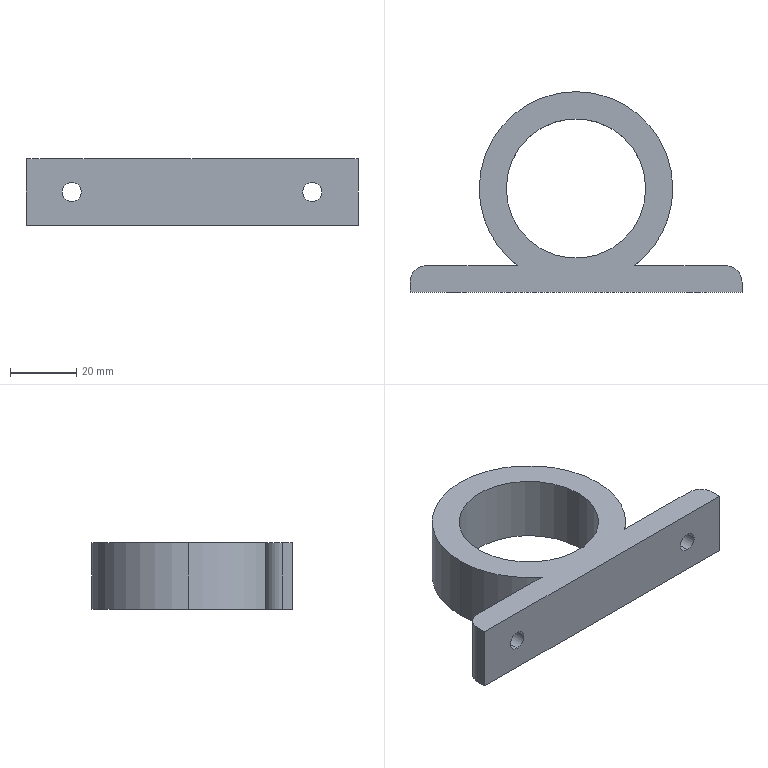Part | SolidWorks | features ICE 3, Extrusion 1, Fillet 1 | 1 solid | 18 faces | box 100 x 60.381 x 20 mm | volume 38212 mm3 | cylinder 11 | plane 7 | commonest cylinder face diameters 5.8 x4 58.309 x3 10 x2 42 x2
STEP:
#1=CARTESIAN_POINT('',(-21.,31.226,-10.));
#2=VERTEX_POINT('',#1);
#3=CARTESIAN_POINT('',(21.,31.226,-10.));
#4=VERTEX_POINT('',#3);
#5=CARTESIAN_POINT('',(0.,31.226,-10.));
#6=DIRECTION('',(0.,0.,1.));
#7=DIRECTION('',(1.,0.,0.));
#8=AXIS2_PLACEMENT_3D('',#5,#6,#7);
#9=CIRCLE('',#8,21.);
#10=EDGE_CURVE('',#2,#4,#9,.T.);
#11=ORIENTED_EDGE('',*,*,#10,.F.);
#12=CARTESIAN_POINT('',(-21.,31.226,10.));
#13=VERTEX_POINT('',#12);
#14=CARTESIAN_POINT('',(-21.,31.226,-64.));
#15=DIRECTION('',(0.,0.,1.));
#16=VECTOR('',#15,1000.);
#17=LINE('',#14,#16);
#18=EDGE_CURVE('',#2,#13,#17,.T.);
#19=ORIENTED_EDGE('',*,*,#18,.T.);
#20=CARTESIAN_POINT('',(21.,31.226,10.));
#21=VERTEX_POINT('',#20);
#22=CARTESIAN_POINT('',(0.,31.226,10.));
#23=DIRECTION('',(0.,0.,1.));
#24=DIRECTION('',(1.,0.,0.));
#25=AXIS2_PLACEMENT_3D('',#22,#23,#24);
#26=CIRCLE('',#25,21.);
#27=EDGE_CURVE('',#13,#21,#26,.T.);
#28=ORIENTED_EDGE('',*,*,#27,.T.);
#29=CARTESIAN_POINT('',(21.,31.226,-64.));
#30=DIRECTION('',(0.,0.,1.));
#31=VECTOR('',#30,1000.);
#32=LINE('',#29,#31);
#33=EDGE_CURVE('',#4,#21,#32,.T.);
#34=ORIENTED_EDGE('',*,*,#33,.F.);
#35=EDGE_LOOP('',(#11,#19,#28,#34));
#36=FACE_OUTER_BOUND('',#35,.T.);
#37=CARTESIAN_POINT('',(0.,31.226,-64.));
#38=DIRECTION('',(0.,0.,1.));
#39=DIRECTION('',(1.,0.,0.));
#40=AXIS2_PLACEMENT_3D('',#37,#38,#39);
#41=CYLINDRICAL_SURFACE('',#40,21.);
#42=ADVANCED_FACE('',(#36),#41,.F.);
#43=CARTESIAN_POINT('',(-36.247,0.,-2.9));
#44=VERTEX_POINT('',#43);
#45=CARTESIAN_POINT('',(-36.247,0.,2.9));
#46=VERTEX_POINT('',#45);
#47=CARTESIAN_POINT('',(-36.247,0.,0.));
#48=DIRECTION('',(0.,1.,0.));
#49=DIRECTION('',(0.,0.,1.));
#50=AXIS2_PLACEMENT_3D('',#47,#48,#49);
#51=CIRCLE('',#50,2.9);
#52=EDGE_CURVE('',#44,#46,#51,.T.);
#53=ORIENTED_EDGE('',*,*,#52,.F.);
#54=CARTESIAN_POINT('',(-36.247,8.,-2.9));
#55=VERTEX_POINT('',#54);
#56=CARTESIAN_POINT('',(-36.247,-18.,-2.9));
#57=DIRECTION('',(0.,1.,0.));
#58=VECTOR('',#57,1000.);
#59=LINE('',#56,#58);
#60=EDGE_CURVE('',#44,#55,#59,.T.);
#61=ORIENTED_EDGE('',*,*,#60,.T.);
#62=CARTESIAN_POINT('',(-36.247,8.,2.9));
#63=VERTEX_POINT('',#62);
#64=CARTESIAN_POINT('',(-36.247,8.,0.));
#65=DIRECTION('',(0.,1.,0.));
#66=DIRECTION('',(0.,0.,1.));
#67=AXIS2_PLACEMENT_3D('',#64,#65,#66);
#68=CIRCLE('',#67,2.9);
#69=EDGE_CURVE('',#55,#63,#68,.T.);
#70=ORIENTED_EDGE('',*,*,#69,.T.);
#71=CARTESIAN_POINT('',(-36.247,-18.,2.9));
#72=DIRECTION('',(0.,1.,0.));
#73=VECTOR('',#72,1000.);
#74=LINE('',#71,#73);
#75=EDGE_CURVE('',#46,#63,#74,.T.);
#76=ORIENTED_EDGE('',*,*,#75,.F.);
#77=EDGE_LOOP('',(#53,#61,#70,#76));
#78=FACE_OUTER_BOUND('',#77,.T.);
#79=CARTESIAN_POINT('',(-36.247,-18.,0.));
#80=DIRECTION('',(0.,1.,0.));
#81=DIRECTION('',(0.,0.,1.));
#82=AXIS2_PLACEMENT_3D('',#79,#80,#81);
#83=CYLINDRICAL_SURFACE('',#82,2.9);
#84=ADVANCED_FACE('',(#78),#83,.F.);
#85=CARTESIAN_POINT('',(36.247,0.,-2.9));
#86=VERTEX_POINT('',#85);
#87=CARTESIAN_POINT('',(36.247,0.,2.9));
#88=VERTEX_POINT('',#87);
#89=CARTESIAN_POINT('',(36.247,0.,0.));
#90=DIRECTION('',(0.,1.,0.));
#91=DIRECTION('',(0.,0.,1.));
#92=AXIS2_PLACEMENT_3D('',#89,#90,#91);
#93=CIRCLE('',#92,2.9);
#94=EDGE_CURVE('',#86,#88,#93,.T.);
#95=ORIENTED_EDGE('',*,*,#94,.F.);
#96=CARTESIAN_POINT('',(36.247,8.,-2.9));
#97=VERTEX_POINT('',#96);
#98=CARTESIAN_POINT('',(36.247,-18.,-2.9));
#99=DIRECTION('',(0.,1.,0.));
#100=VECTOR('',#99,1000.);
#101=LINE('',#98,#100);
#102=EDGE_CURVE('',#86,#97,#101,.T.);
#103=ORIENTED_EDGE('',*,*,#102,.T.);
#104=CARTESIAN_POINT('',(36.247,8.,2.9));
#105=VERTEX_POINT('',#104);
#106=CARTESIAN_POINT('',(36.247,8.,0.));
#107=DIRECTION('',(0.,1.,0.));
#108=DIRECTION('',(0.,0.,-1.));
#109=AXIS2_PLACEMENT_3D('',#106,#107,#108);
#110=CIRCLE('',#109,2.9);
#111=EDGE_CURVE('',#97,#105,#110,.T.);
#112=ORIENTED_EDGE('',*,*,#111,.T.);
#113=CARTESIAN_POINT('',(36.247,-18.,2.9));
#114=DIRECTION('',(0.,1.,0.));
#115=VECTOR('',#114,1000.);
#116=LINE('',#113,#115);
#117=EDGE_CURVE('',#88,#105,#116,.T.);
#118=ORIENTED_EDGE('',*,*,#117,.F.);
#119=EDGE_LOOP('',(#95,#103,#112,#118));
#120=FACE_OUTER_BOUND('',#119,.T.);
#121=CARTESIAN_POINT('',(36.247,-18.,0.));
#122=DIRECTION('',(0.,1.,0.));
#123=DIRECTION('',(0.,0.,1.));
#124=AXIS2_PLACEMENT_3D('',#121,#122,#123);
#125=CYLINDRICAL_SURFACE('',#124,2.9);
#126=ADVANCED_FACE('',(#120),#125,.F.);
#127=CARTESIAN_POINT('',(-29.154,31.226,-10.));
#128=VERTEX_POINT('',#127);
#129=CARTESIAN_POINT('',(29.154,31.226,-10.));
#130=VERTEX_POINT('',#129);
#131=CARTESIAN_POINT('',(0.,31.226,-10.));
#132=DIRECTION('',(0.,0.,-1.));
#133=DIRECTION('',(1.,0.,0.));
#134=AXIS2_PLACEMENT_3D('',#131,#132,#133);
#135=CIRCLE('',#134,29.154);
#136=EDGE_CURVE('',#128,#130,#135,.T.);
#137=ORIENTED_EDGE('',*,*,#136,.F.);
#138=CARTESIAN_POINT('',(-29.154,31.226,10.));
#139=VERTEX_POINT('',#138);
#140=CARTESIAN_POINT('',(-29.154,31.226,-126.815));
#141=DIRECTION('',(0.,0.,1.));
#142=VECTOR('',#141,1000.);
#143=LINE('',#140,#142);
#144=EDGE_CURVE('',#128,#139,#143,.T.);
#145=ORIENTED_EDGE('',*,*,#144,.T.);
#146=CARTESIAN_POINT('',(29.154,31.226,10.));
#147=VERTEX_POINT('',#146);
#148=CARTESIAN_POINT('',(0.,31.226,10.));
#149=DIRECTION('',(0.,0.,1.));
#150=DIRECTION('',(1.,0.,0.));
#151=AXIS2_PLACEMENT_3D('',#148,#149,#150);
#152=CIRCLE('',#151,29.154);
#153=EDGE_CURVE('',#147,#139,#152,.T.);
#154=ORIENTED_EDGE('',*,*,#153,.F.);
#155=CARTESIAN_POINT('',(29.154,31.226,-126.815));
#156=DIRECTION('',(0.,0.,1.));
#157=VECTOR('',#156,1000.);
#158=LINE('',#155,#157);
#159=EDGE_CURVE('',#130,#147,#158,.T.);
#160=ORIENTED_EDGE('',*,*,#159,.F.);
#161=EDGE_LOOP('',(#137,#145,#154,#160));
#162=FACE_OUTER_BOUND('',#161,.T.);
#163=CARTESIAN_POINT('',(0.,31.226,-126.815));
#164=DIRECTION('',(0.,0.,1.));
#165=DIRECTION('',(1.,0.,0.));
#166=AXIS2_PLACEMENT_3D('',#163,#164,#165);
#167=CYLINDRICAL_SURFACE('',#166,29.154);
#168=ADVANCED_FACE('',(#162),#167,.T.);
#169=CARTESIAN_POINT('',(17.621,8.,-10.));
#170=VERTEX_POINT('',#169);
#171=CARTESIAN_POINT('',(0.,31.226,-10.));
#172=DIRECTION('',(0.,0.,-1.));
#173=DIRECTION('',(1.,0.,0.));
#174=AXIS2_PLACEMENT_3D('',#171,#172,#173);
#175=CIRCLE('',#174,29.154);
#176=EDGE_CURVE('',#130,#170,#175,.T.);
#177=ORIENTED_EDGE('',*,*,#176,.F.);
#178=ORIENTED_EDGE('',*,*,#159,.T.);
#179=CARTESIAN_POINT('',(17.621,8.,10.));
#180=VERTEX_POINT('',#179);
#181=CARTESIAN_POINT('',(0.,31.226,10.));
#182=DIRECTION('',(0.,0.,1.));
#183=DIRECTION('',(1.,0.,0.));
#184=AXIS2_PLACEMENT_3D('',#181,#182,#183);
#185=CIRCLE('',#184,29.154);
#186=EDGE_CURVE('',#180,#147,#185,.T.);
#187=ORIENTED_EDGE('',*,*,#186,.F.);
#188=CARTESIAN_POINT('',(17.621,8.,-126.815));
#189=DIRECTION('',(0.,0.,1.));
#190=VECTOR('',#189,1000.);
#191=LINE('',#188,#190);
#192=EDGE_CURVE('',#170,#180,#191,.T.);
#193=ORIENTED_EDGE('',*,*,#192,.F.);
#194=EDGE_LOOP('',(#177,#178,#187,#193));
#195=FACE_OUTER_BOUND('',#194,.T.);
#196=CARTESIAN_POINT('',(0.,31.226,-126.815));
#197=DIRECTION('',(0.,0.,1.));
#198=DIRECTION('',(1.,0.,0.));
#199=AXIS2_PLACEMENT_3D('',#196,#197,#198);
#200=CYLINDRICAL_SURFACE('',#199,29.154);
#201=ADVANCED_FACE('',(#195),#200,.T.);
#202=CARTESIAN_POINT('',(-36.247,8.,0.));
#203=DIRECTION('',(0.,1.,0.));
#204=DIRECTION('',(0.,0.,1.));
#205=AXIS2_PLACEMENT_3D('',#202,#203,#204);
#206=CIRCLE('',#205,2.9);
#207=EDGE_CURVE('',#63,#55,#206,.T.);
#208=ORIENTED_EDGE('',*,*,#207,.F.);
#209=ORIENTED_EDGE('',*,*,#69,.F.);
#210=EDGE_LOOP('',(#208,#209));
#211=FACE_BOUND('',#210,.T.);
#212=CARTESIAN_POINT('',(-17.621,8.,-10.));
#213=VERTEX_POINT('',#212);
#214=CARTESIAN_POINT('',(-17.621,8.,10.));
#215=VERTEX_POINT('',#214);
#216=CARTESIAN_POINT('',(-17.621,8.,-126.815));
#217=DIRECTION('',(0.,0.,1.));
#218=VECTOR('',#217,1000.);
#219=LINE('',#216,#218);
#220=EDGE_CURVE('',#213,#215,#219,.T.);
#221=ORIENTED_EDGE('',*,*,#220,.F.);
#222=CARTESIAN_POINT('',(-45.,8.,-10.));
#223=VERTEX_POINT('',#222);
#224=CARTESIAN_POINT('',(-50.,8.,-10.));
#225=DIRECTION('',(-1.,0.,0.));
#226=VECTOR('',#225,1000.);
#227=LINE('',#224,#226);
#228=EDGE_CURVE('',#213,#223,#227,.T.);
#229=ORIENTED_EDGE('',*,*,#228,.T.);
#230=CARTESIAN_POINT('',(-45.,8.,10.));
#231=VERTEX_POINT('',#230);
#232=CARTESIAN_POINT('',(-45.,8.,10.));
#233=DIRECTION('',(0.,0.,1.));
#234=VECTOR('',#233,1000.);
#235=LINE('',#232,#234);
#236=EDGE_CURVE('',#223,#231,#235,.T.);
#237=ORIENTED_EDGE('',*,*,#236,.T.);
#238=CARTESIAN_POINT('',(-50.,8.,10.));
#239=DIRECTION('',(1.,0.,0.));
#240=VECTOR('',#239,1000.);
#241=LINE('',#238,#240);
#242=EDGE_CURVE('',#231,#215,#241,.T.);
#243=ORIENTED_EDGE('',*,*,#242,.T.);
#244=EDGE_LOOP('',(#221,#229,#237,#243));
#245=FACE_OUTER_BOUND('',#244,.T.);
#246=CARTESIAN_POINT('',(0.,8.,0.));
#247=DIRECTION('',(0.,1.,0.));
#248=DIRECTION('',(0.,0.,1.));
#249=AXIS2_PLACEMENT_3D('',#246,#247,#248);
#250=PLANE('',#249);
#251=ADVANCED_FACE('',(#211,#245),#250,.T.);
#252=CARTESIAN_POINT('',(50.,3.,-10.));
#253=VERTEX_POINT('',#252);
#254=CARTESIAN_POINT('',(50.,0.,-10.));
#255=VERTEX_POINT('',#254);
#256=CARTESIAN_POINT('',(50.,8.,-10.));
#257=DIRECTION('',(0.,-1.,0.));
#258=VECTOR('',#257,1000.);
#259=LINE('',#256,#258);
#260=EDGE_CURVE('',#253,#255,#259,.T.);
#261=ORIENTED_EDGE('',*,*,#260,.F.);
#262=CARTESIAN_POINT('',(50.,3.,10.));
#263=VERTEX_POINT('',#262);
#264=CARTESIAN_POINT('',(50.,3.,10.));
#265=DIRECTION('',(0.,0.,1.));
#266=VECTOR('',#265,1000.);
#267=LINE('',#264,#266);
#268=EDGE_CURVE('',#253,#263,#267,.T.);
#269=ORIENTED_EDGE('',*,*,#268,.T.);
#270=CARTESIAN_POINT('',(50.,0.,10.));
#271=VERTEX_POINT('',#270);
#272=CARTESIAN_POINT('',(50.,8.,10.));
#273=DIRECTION('',(0.,-1.,0.));
#274=VECTOR('',#273,1000.);
#275=LINE('',#272,#274);
#276=EDGE_CURVE('',#263,#271,#275,.T.);
#277=ORIENTED_EDGE('',*,*,#276,.T.);
#278=CARTESIAN_POINT('',(50.,0.,-10.));
#279=DIRECTION('',(0.,0.,-1.));
#280=VECTOR('',#279,1000.);
#281=LINE('',#278,#280);
#282=EDGE_CURVE('',#271,#255,#281,.T.);
#283=ORIENTED_EDGE('',*,*,#282,.T.);
#284=EDGE_LOOP('',(#261,#269,#277,#283));
#285=FACE_OUTER_BOUND('',#284,.T.);
#286=CARTESIAN_POINT('',(50.,8.,-10.));
#287=DIRECTION('',(-1.,0.,0.));
#288=DIRECTION('',(0.,0.,1.));
#289=AXIS2_PLACEMENT_3D('',#286,#287,#288);
#290=PLANE('',#289);
#291=ADVANCED_FACE('',(#285),#290,.F.);
#292=CARTESIAN_POINT('',(0.,31.226,-10.));
#293=DIRECTION('',(0.,0.,1.));
#294=DIRECTION('',(1.,0.,0.));
#295=AXIS2_PLACEMENT_3D('',#292,#293,#294);
#296=CIRCLE('',#295,21.);
#297=EDGE_CURVE('',#4,#2,#296,.T.);
#298=ORIENTED_EDGE('',*,*,#297,.T.);
#299=ORIENTED_EDGE('',*,*,#10,.T.);
#300=EDGE_LOOP('',(#298,#299));
#301=FACE_BOUND('',#300,.T.);
#302=CARTESIAN_POINT('',(-50.,3.,-10.));
#303=VERTEX_POINT('',#302);
#304=CARTESIAN_POINT('',(-50.,0.,-10.));
#305=VERTEX_POINT('',#304);
#306=CARTESIAN_POINT('',(-50.,8.,-10.));
#307=DIRECTION('',(0.,-1.,0.));
#308=VECTOR('',#307,1000.);
#309=LINE('',#306,#308);
#310=EDGE_CURVE('',#303,#305,#309,.T.);
#311=ORIENTED_EDGE('',*,*,#310,.F.);
#312=CARTESIAN_POINT('',(-45.,3.,-10.));
#313=DIRECTION('',(0.,0.,-1.));
#314=DIRECTION('',(1.,0.,0.));
#315=AXIS2_PLACEMENT_3D('',#312,#313,#314);
#316=CIRCLE('',#315,5.);
#317=EDGE_CURVE('',#303,#223,#316,.T.);
#318=ORIENTED_EDGE('',*,*,#317,.T.);
#319=ORIENTED_EDGE('',*,*,#228,.F.);
#320=CARTESIAN_POINT('',(0.,31.226,-10.));
#321=DIRECTION('',(0.,0.,-1.));
#322=DIRECTION('',(1.,0.,0.));
#323=AXIS2_PLACEMENT_3D('',#320,#321,#322);
#324=CIRCLE('',#323,29.154);
#325=EDGE_CURVE('',#213,#128,#324,.T.);
#326=ORIENTED_EDGE('',*,*,#325,.T.);
#327=ORIENTED_EDGE('',*,*,#136,.T.);
#328=ORIENTED_EDGE('',*,*,#176,.T.);
#329=CARTESIAN_POINT('',(45.,8.,-10.));
#330=VERTEX_POINT('',#329);
#331=CARTESIAN_POINT('',(-50.,8.,-10.));
#332=DIRECTION('',(-1.,0.,0.));
#333=VECTOR('',#332,1000.);
#334=LINE('',#331,#333);
#335=EDGE_CURVE('',#330,#170,#334,.T.);
#336=ORIENTED_EDGE('',*,*,#335,.F.);
#337=CARTESIAN_POINT('',(45.,3.,-10.));
#338=DIRECTION('',(0.,0.,-1.));
#339=DIRECTION('',(1.,0.,0.));
#340=AXIS2_PLACEMENT_3D('',#337,#338,#339);
#341=CIRCLE('',#340,5.);
#342=EDGE_CURVE('',#330,#253,#341,.T.);
#343=ORIENTED_EDGE('',*,*,#342,.T.);
#344=ORIENTED_EDGE('',*,*,#260,.T.);
#345=CARTESIAN_POINT('',(-50.,0.,-10.));
#346=DIRECTION('',(-1.,0.,0.));
#347=VECTOR('',#346,1000.);
#348=LINE('',#345,#347);
#349=EDGE_CURVE('',#255,#305,#348,.T.);
#350=ORIENTED_EDGE('',*,*,#349,.T.);
#351=EDGE_LOOP('',(#311,#318,#319,#326,#327,#328,#336,#343,#344,#350));
#352=FACE_OUTER_BOUND('',#351,.T.);
#353=CARTESIAN_POINT('',(-50.,8.,-10.));
#354=DIRECTION('',(0.,0.,1.));
#355=DIRECTION('',(1.,0.,0.));
#356=AXIS2_PLACEMENT_3D('',#353,#354,#355);
#357=PLANE('',#356);
#358=ADVANCED_FACE('',(#301,#352),#357,.F.);
#359=CARTESIAN_POINT('',(-50.,3.,10.));
#360=VERTEX_POINT('',#359);
#361=CARTESIAN_POINT('',(-50.,0.,10.));
#362=VERTEX_POINT('',#361);
#363=CARTESIAN_POINT('',(-50.,8.,10.));
#364=DIRECTION('',(0.,-1.,0.));
#365=VECTOR('',#364,1000.);
#366=LINE('',#363,#365);
#367=EDGE_CURVE('',#360,#362,#366,.T.);
#368=ORIENTED_EDGE('',*,*,#367,.F.);
#369=CARTESIAN_POINT('',(-50.,3.,-10.));
#370=DIRECTION('',(0.,0.,-1.));
#371=VECTOR('',#370,1000.);
#372=LINE('',#369,#371);
#373=EDGE_CURVE('',#360,#303,#372,.T.);
#374=ORIENTED_EDGE('',*,*,#373,.T.);
#375=ORIENTED_EDGE('',*,*,#310,.T.);
#376=CARTESIAN_POINT('',(-50.,0.,-10.));
#377=DIRECTION('',(0.,0.,1.));
#378=VECTOR('',#377,1000.);
#379=LINE('',#376,#378);
#380=EDGE_CURVE('',#305,#362,#379,.T.);
#381=ORIENTED_EDGE('',*,*,#380,.T.);
#382=EDGE_LOOP('',(#368,#374,#375,#381));
#383=FACE_OUTER_BOUND('',#382,.T.);
#384=CARTESIAN_POINT('',(-50.,8.,-10.));
#385=DIRECTION('',(1.,0.,0.));
#386=DIRECTION('',(0.,0.,-1.));
#387=AXIS2_PLACEMENT_3D('',#384,#385,#386);
#388=PLANE('',#387);
#389=ADVANCED_FACE('',(#383),#388,.F.);
#390=CARTESIAN_POINT('',(0.,31.226,10.));
#391=DIRECTION('',(0.,0.,1.));
#392=DIRECTION('',(1.,0.,0.));
#393=AXIS2_PLACEMENT_3D('',#390,#391,#392);
#394=CIRCLE('',#393,21.);
#395=EDGE_CURVE('',#21,#13,#394,.T.);
#396=ORIENTED_EDGE('',*,*,#395,.F.);
#397=ORIENTED_EDGE('',*,*,#27,.F.);
#398=EDGE_LOOP('',(#396,#397));
#399=FACE_BOUND('',#398,.T.);
#400=ORIENTED_EDGE('',*,*,#242,.F.);
#401=CARTESIAN_POINT('',(-45.,3.,10.));
#402=DIRECTION('',(0.,0.,1.));
#403=DIRECTION('',(-1.,0.,0.));
#404=AXIS2_PLACEMENT_3D('',#401,#402,#403);
#405=CIRCLE('',#404,5.);
#406=EDGE_CURVE('',#231,#360,#405,.T.);
#407=ORIENTED_EDGE('',*,*,#406,.T.);
#408=ORIENTED_EDGE('',*,*,#367,.T.);
#409=CARTESIAN_POINT('',(-50.,0.,10.));
#410=DIRECTION('',(1.,0.,0.));
#411=VECTOR('',#410,1000.);
#412=LINE('',#409,#411);
#413=EDGE_CURVE('',#362,#271,#412,.T.);
#414=ORIENTED_EDGE('',*,*,#413,.T.);
#415=ORIENTED_EDGE('',*,*,#276,.F.);
#416=CARTESIAN_POINT('',(45.,8.,10.));
#417=VERTEX_POINT('',#416);
#418=CARTESIAN_POINT('',(45.,3.,10.));
#419=DIRECTION('',(0.,0.,1.));
#420=DIRECTION('',(-1.,0.,0.));
#421=AXIS2_PLACEMENT_3D('',#418,#419,#420);
#422=CIRCLE('',#421,5.);
#423=EDGE_CURVE('',#263,#417,#422,.T.);
#424=ORIENTED_EDGE('',*,*,#423,.T.);
#425=CARTESIAN_POINT('',(-50.,8.,10.));
#426=DIRECTION('',(1.,0.,0.));
#427=VECTOR('',#426,1000.);
#428=LINE('',#425,#427);
#429=EDGE_CURVE('',#180,#417,#428,.T.);
#430=ORIENTED_EDGE('',*,*,#429,.F.);
#431=ORIENTED_EDGE('',*,*,#186,.T.);
#432=ORIENTED_EDGE('',*,*,#153,.T.);
#433=CARTESIAN_POINT('',(0.,31.226,10.));
#434=DIRECTION('',(0.,0.,1.));
#435=DIRECTION('',(1.,0.,0.));
#436=AXIS2_PLACEMENT_3D('',#433,#434,#435);
#437=CIRCLE('',#436,29.154);
#438=EDGE_CURVE('',#139,#215,#437,.T.);
#439=ORIENTED_EDGE('',*,*,#438,.T.);
#440=EDGE_LOOP('',(#400,#407,#408,#414,#415,#424,#430,#431,#432,#439));
#441=FACE_OUTER_BOUND('',#440,.T.);
#442=CARTESIAN_POINT('',(-50.,8.,10.));
#443=DIRECTION('',(0.,0.,-1.));
#444=DIRECTION('',(-1.,0.,0.));
#445=AXIS2_PLACEMENT_3D('',#442,#443,#444);
#446=PLANE('',#445);
#447=ADVANCED_FACE('',(#399,#441),#446,.F.);
#448=CARTESIAN_POINT('',(36.247,8.,0.));
#449=DIRECTION('',(0.,1.,0.));
#450=DIRECTION('',(0.,0.,-1.));
#451=AXIS2_PLACEMENT_3D('',#448,#449,#450);
#452=CIRCLE('',#451,2.9);
#453=EDGE_CURVE('',#105,#97,#452,.T.);
#454=ORIENTED_EDGE('',*,*,#453,.F.);
#455=ORIENTED_EDGE('',*,*,#111,.F.);
#456=EDGE_LOOP('',(#454,#455));
#457=FACE_BOUND('',#456,.T.);
#458=ORIENTED_EDGE('',*,*,#192,.T.);
#459=ORIENTED_EDGE('',*,*,#429,.T.);
#460=CARTESIAN_POINT('',(45.,8.,-10.));
#461=DIRECTION('',(0.,0.,-1.));
#462=VECTOR('',#461,1000.);
#463=LINE('',#460,#462);
#464=EDGE_CURVE('',#417,#330,#463,.T.);
#465=ORIENTED_EDGE('',*,*,#464,.T.);
#466=ORIENTED_EDGE('',*,*,#335,.T.);
#467=EDGE_LOOP('',(#458,#459,#465,#466));
#468=FACE_OUTER_BOUND('',#467,.T.);
#469=CARTESIAN_POINT('',(0.,8.,0.));
#470=DIRECTION('',(0.,1.,0.));
#471=DIRECTION('',(0.,0.,1.));
#472=AXIS2_PLACEMENT_3D('',#469,#470,#471);
#473=PLANE('',#472);
#474=ADVANCED_FACE('',(#457,#468),#473,.T.);
#475=CARTESIAN_POINT('',(-36.247,0.,0.));
#476=DIRECTION('',(0.,1.,0.));
#477=DIRECTION('',(0.,0.,1.));
#478=AXIS2_PLACEMENT_3D('',#475,#476,#477);
#479=CIRCLE('',#478,2.9);
#480=EDGE_CURVE('',#46,#44,#479,.T.);
#481=ORIENTED_EDGE('',*,*,#480,.T.);
#482=ORIENTED_EDGE('',*,*,#52,.T.);
#483=EDGE_LOOP('',(#481,#482));
#484=FACE_BOUND('',#483,.T.);
#485=CARTESIAN_POINT('',(36.247,0.,0.));
#486=DIRECTION('',(0.,1.,0.));
#487=DIRECTION('',(0.,0.,1.));
#488=AXIS2_PLACEMENT_3D('',#485,#486,#487);
#489=CIRCLE('',#488,2.9);
#490=EDGE_CURVE('',#88,#86,#489,.T.);
#491=ORIENTED_EDGE('',*,*,#490,.T.);
#492=ORIENTED_EDGE('',*,*,#94,.T.);
#493=EDGE_LOOP('',(#491,#492));
#494=FACE_BOUND('',#493,.T.);
#495=ORIENTED_EDGE('',*,*,#282,.F.);
#496=ORIENTED_EDGE('',*,*,#413,.F.);
#497=ORIENTED_EDGE('',*,*,#380,.F.);
#498=ORIENTED_EDGE('',*,*,#349,.F.);
#499=EDGE_LOOP('',(#495,#496,#497,#498));
#500=FACE_OUTER_BOUND('',#499,.T.);
#501=CARTESIAN_POINT('',(0.,0.,0.));
#502=DIRECTION('',(0.,1.,0.));
#503=DIRECTION('',(0.,0.,1.));
#504=AXIS2_PLACEMENT_3D('',#501,#502,#503);
#505=PLANE('',#504);
#506=ADVANCED_FACE('',(#484,#494,#500),#505,.F.);
#507=ORIENTED_EDGE('',*,*,#317,.F.);
#508=ORIENTED_EDGE('',*,*,#373,.F.);
#509=ORIENTED_EDGE('',*,*,#406,.F.);
#510=ORIENTED_EDGE('',*,*,#236,.F.);
#511=EDGE_LOOP('',(#507,#508,#509,#510));
#512=FACE_OUTER_BOUND('',#511,.T.);
#513=CARTESIAN_POINT('',(-45.,3.,0.));
#514=DIRECTION('',(0.,0.,-1.));
#515=DIRECTION('',(-1.,0.,0.));
#516=AXIS2_PLACEMENT_3D('',#513,#514,#515);
#517=CYLINDRICAL_SURFACE('',#516,5.);
#518=ADVANCED_FACE('',(#512),#517,.T.);
#519=ORIENTED_EDGE('',*,*,#423,.F.);
#520=ORIENTED_EDGE('',*,*,#268,.F.);
#521=ORIENTED_EDGE('',*,*,#342,.F.);
#522=ORIENTED_EDGE('',*,*,#464,.F.);
#523=EDGE_LOOP('',(#519,#520,#521,#522));
#524=FACE_OUTER_BOUND('',#523,.T.);
#525=CARTESIAN_POINT('',(45.,3.,0.));
#526=DIRECTION('',(0.,0.,1.));
#527=DIRECTION('',(1.,0.,0.));
#528=AXIS2_PLACEMENT_3D('',#525,#526,#527);
#529=CYLINDRICAL_SURFACE('',#528,5.);
#530=ADVANCED_FACE('',(#524),#529,.T.);
#531=ORIENTED_EDGE('',*,*,#144,.F.);
#532=ORIENTED_EDGE('',*,*,#325,.F.);
#533=ORIENTED_EDGE('',*,*,#220,.T.);
#534=ORIENTED_EDGE('',*,*,#438,.F.);
#535=EDGE_LOOP('',(#531,#532,#533,#534));
#536=FACE_OUTER_BOUND('',#535,.T.);
#537=CARTESIAN_POINT('',(0.,31.226,-126.815));
#538=DIRECTION('',(0.,0.,1.));
#539=DIRECTION('',(1.,0.,0.));
#540=AXIS2_PLACEMENT_3D('',#537,#538,#539);
#541=CYLINDRICAL_SURFACE('',#540,29.154);
#542=ADVANCED_FACE('',(#536),#541,.T.);
#543=ORIENTED_EDGE('',*,*,#102,.F.);
#544=ORIENTED_EDGE('',*,*,#490,.F.);
#545=ORIENTED_EDGE('',*,*,#117,.T.);
#546=ORIENTED_EDGE('',*,*,#453,.T.);
#547=EDGE_LOOP('',(#543,#544,#545,#546));
#548=FACE_OUTER_BOUND('',#547,.T.);
#549=CARTESIAN_POINT('',(36.247,-18.,0.));
#550=DIRECTION('',(0.,1.,0.));
#551=DIRECTION('',(0.,0.,1.));
#552=AXIS2_PLACEMENT_3D('',#549,#550,#551);
#553=CYLINDRICAL_SURFACE('',#552,2.9);
#554=ADVANCED_FACE('',(#548),#553,.F.);
#555=ORIENTED_EDGE('',*,*,#60,.F.);
#556=ORIENTED_EDGE('',*,*,#480,.F.);
#557=ORIENTED_EDGE('',*,*,#75,.T.);
#558=ORIENTED_EDGE('',*,*,#207,.T.);
#559=EDGE_LOOP('',(#555,#556,#557,#558));
#560=FACE_OUTER_BOUND('',#559,.T.);
#561=CARTESIAN_POINT('',(-36.247,-18.,0.));
#562=DIRECTION('',(0.,1.,0.));
#563=DIRECTION('',(0.,0.,1.));
#564=AXIS2_PLACEMENT_3D('',#561,#562,#563);
#565=CYLINDRICAL_SURFACE('',#564,2.9);
#566=ADVANCED_FACE('',(#560),#565,.F.);
#567=ORIENTED_EDGE('',*,*,#18,.F.);
#568=ORIENTED_EDGE('',*,*,#297,.F.);
#569=ORIENTED_EDGE('',*,*,#33,.T.);
#570=ORIENTED_EDGE('',*,*,#395,.T.);
#571=EDGE_LOOP('',(#567,#568,#569,#570));
#572=FACE_OUTER_BOUND('',#571,.T.);
#573=CARTESIAN_POINT('',(0.,31.226,-64.));
#574=DIRECTION('',(0.,0.,1.));
#575=DIRECTION('',(1.,0.,0.));
#576=AXIS2_PLACEMENT_3D('',#573,#574,#575);
#577=CYLINDRICAL_SURFACE('',#576,21.);
#578=ADVANCED_FACE('',(#572),#577,.F.);
#579=CLOSED_SHELL('',(#42,#84,#126,#168,#201,#251,#291,#358,#389,#447,#474,#506,#518,#530,#542,#554,#566,#578));
#580=MANIFOLD_SOLID_BREP('',#579);
#581=CARTESIAN_POINT('',(0.,0.,0.));
#582=DIRECTION('',(0.,0.,1.));
#583=DIRECTION('',(1.,0.,0.));
#584=AXIS2_PLACEMENT_3D('',#581,#582,#583);
#585=(LENGTH_UNIT()NAMED_UNIT(*)SI_UNIT(.MILLI.,.METRE.));
#586=UNCERTAINTY_MEASURE_WITH_UNIT(LENGTH_MEASURE(0.00001),#585,'','');
#587=(NAMED_UNIT(*)PLANE_ANGLE_UNIT()SI_UNIT($,.RADIAN.));
#588=(NAMED_UNIT(*)SI_UNIT($,.STERADIAN.)SOLID_ANGLE_UNIT());
#589=(GEOMETRIC_REPRESENTATION_CONTEXT(3)GLOBAL_UNCERTAINTY_ASSIGNED_CONTEXT((#586))GLOBAL_UNIT_ASSIGNED_CONTEXT((#585,#587,#588))REPRESENTATION_CONTEXT('',''));
#590=ADVANCED_BREP_SHAPE_REPRESENTATION('',(#580,#584),#589);